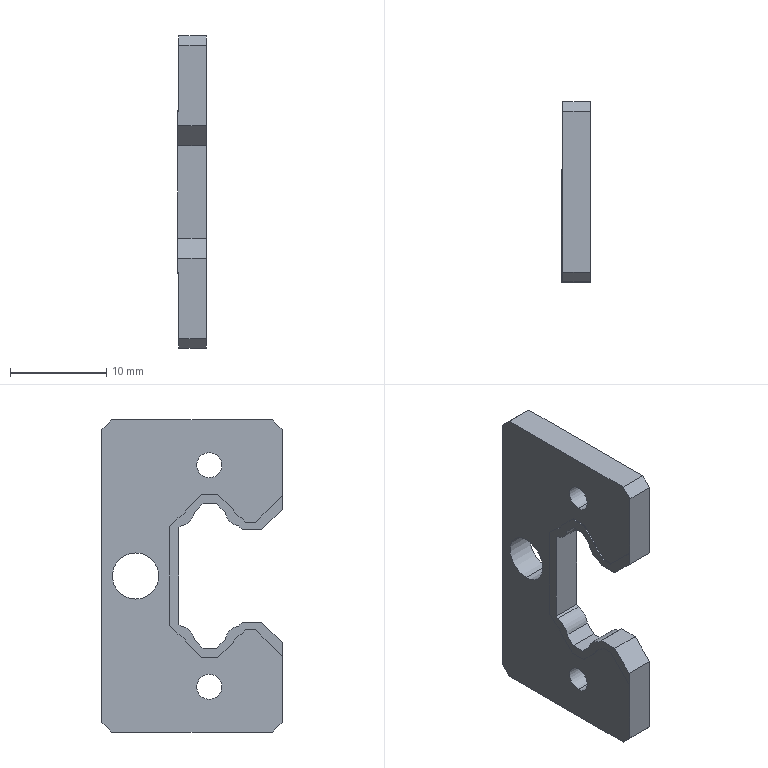Part | STEP file | 920019A1 | 1 solid | 56 faces | box 3 x 18.7 x 32.4 mm | volume 1294 mm3 | plane 42 | cylinder 14 | commonest cylinder face diameters 3.2 x8 2.6 x4 4.8 x2